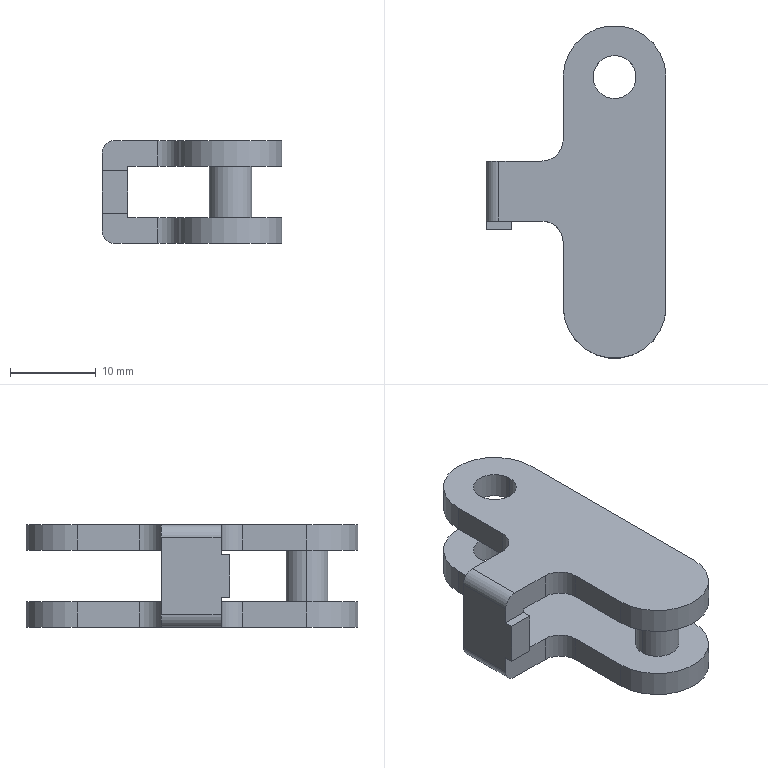Part | STEP file | Sceond_200_APVM0 -3 | 1 solid | 34 faces | box 21 x 38.8 x 12 mm | volume 3137 mm3 | plane 18 | cylinder 16 | commonest cylinder face diameters 5 x10 12 x4 3 x2